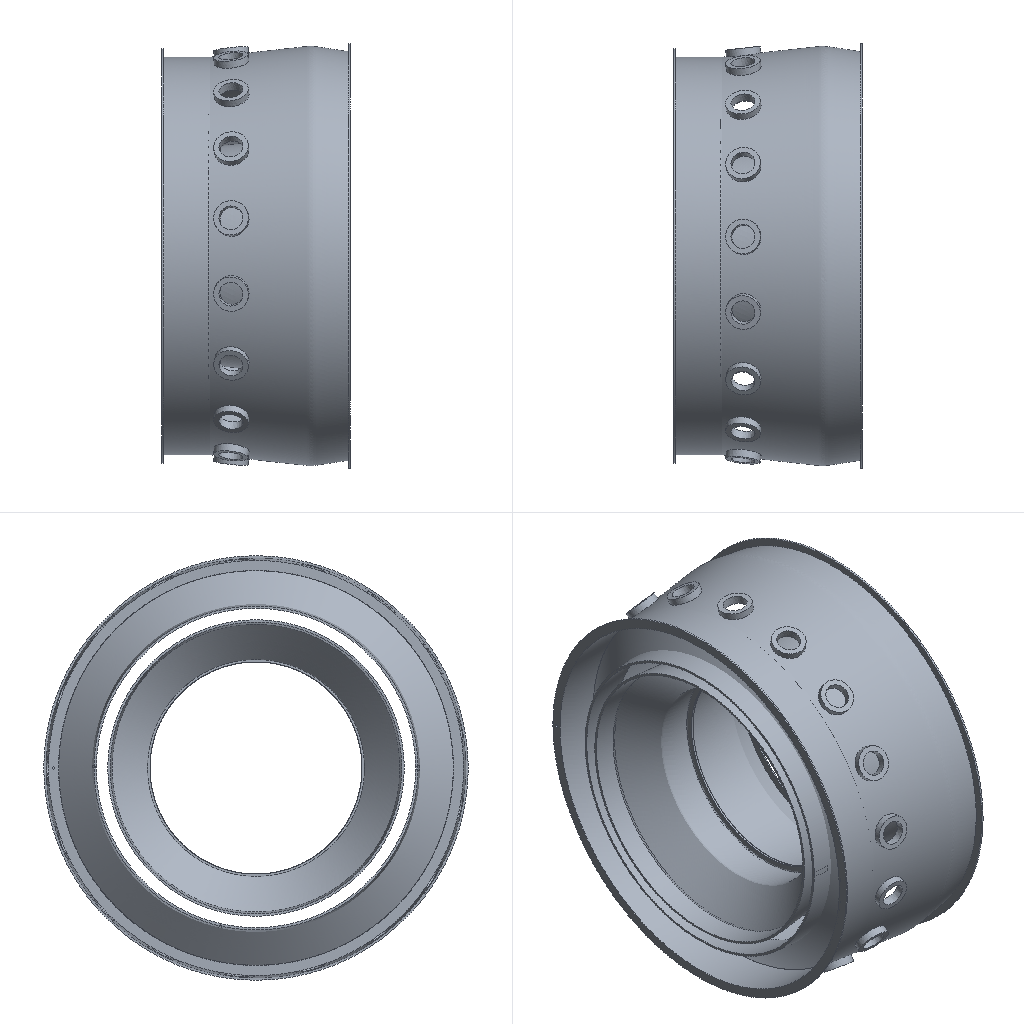Simulation study | ansys workbench
Set-up summary:
category,name,step,type,value,unit,region
solver,ansys_workbench
units,mm-N-s-tonne (MPa),,stated,"/units,MPA"
analysis,LS1,,steady-state thermal
load_step,LS1,LS1,steady-state thermal,nsubst=1; time=1
mesh,nodes,,,1043878
mesh,elements,,,772711
element_type,SOLID291,,,508745
element_type,SURF152,,,252830
element_type,SOLID279,,,6528
element_type,TARGE170,,,2304
element_type,CONTA174,,,2304
material,GH141,,E,216000
material,GH141,,nu,0.31
material,GH141,,density,8.27e-09,tonne mm^-3
material,GH141,,conductivity,8.37
material,GH141,,cte,1.054e-05
load,Define Uniform Initial temperature,model,body load temp,21.85,,all
load,"Create ""______""",LS1,convection,0.05,,SURF152 #8
load,"Create ""______ 2""",LS1,convection,0.288,,SURF152 #9
contact,Contact Region,,bonded (always),element=CONTA174
Ansys APDL input file, long lists of numbers shortened:
/batch
/config,noeldb,1     ! force off writing results to database
*get,_wallstrt,active,,time,wall
! ANSYS input file written by Workbench version 2021 R1
! File used for geometry attach:
/title,____+__+__--___ (B5)
! ****** Begin Custom Load Command Snippet ******
/COM, ACT Extensions:
/COM,     LSDYNA, 2021.1
/COM,
! ****** End   Custom Load Command Snippet ******
*DIM,_wb_ProjectScratch_dir,string,248
_wb_ProjectScratch_dir(1) = ''
*DIM,_wb_SolverFiles_dir,string,248
_wb_SolverFiles_dir(1) = ''
*DIM,_wb_userfiles_dir,string,248
_wb_userfiles_dir(1) = ''
/com,--- Data in consistent NMM units. See Solving Units in the help system for more information.
/units,MPA
/nopr
/wb,file,start              !  signify a WB generated input file
/prep7
! Turn off shape checking because checks already performed inside WB mesher.
! See help system for more information.
SHPP,OFF,,NOWARN
/nolist
etcon,set             ! allow ANSYS to choose best KEYOP's for 180x elements, resets any applicable keyopt to MAPDL defaults
/com,*********** Nodes for the whole assembly ***********
nblock,3,,1148263
(1i9,3e20.9e3)
        1    -2.909328663E+02    -6.564341511E+00     4.578700000E+02
! (1043875 more lines like these left out)
-1
/com,*********** Nodes for all Remote Points ***********
nblock,3
(1i9,3e20.9e3)
  1043877    -7.493286614E+01    -6.564353799E+00     2.143080415E+02
  1043878    -7.493286951E+01    -6.697121594E+00     2.143200000E+02
-1
/wb,elem,start            !  set before creation of elements
/com,*********** Elements for Body 1 "____9.24_\____9.24_" ***********
et,1,291
eblock,19,solid,,320859
(19i9)
        1        1        1        1        0        0        0        0       10        0   194415   420982   429274   496877   520848   545299   607590   545303   545309
! (641717 more lines like these left out)
-1
/com,*********** Elements for Body 2 "____0923_ (1)-0\____0923_ (1)" ***********
et,2,279
eblock,19,solid,,6528
(19i9)
        2        2        2        2        0        0        0        0       20        0        1     1050     1051    13262    13261     7008     7007    13469    13470
! (13055 more lines like these left out)
-1
/com,*********** Elements for Body 3 "______9.22_\______9.22_" ***********
et,3,291
eblock,19,solid,,92984
(19i9)
        3        3        3        3        0        0        0        0       10        0    35420    54545   103924   108327   107989   161558   401449   161564   161563
! (185967 more lines like these left out)
-1
/com,*********** Elements for Body 4 "______9.24_\______9.24_" ***********
et,4,291
eblock,19,solid,,66011
(19i9)
        4        4        3        4        0        0        0        0       10        0   128404    55040   108946   103353   108755   164427   399349   164424   164426
! (132021 more lines like these left out)
-1
/com,*********** Elements for Body 5 "____0923_ (1)\____0923_ (1)" ***********
et,5,291
eblock,19,solid,,28891
(19i9)
        5        5        3        5        0        0        0        0       10        0     6529    48274    97425   107256    48526   115927   382662   115929   115926
! (57781 more lines like these left out)
-1
/wb,elem,end               !  done creating elements
/com,*********** Send User Defined Coordinate System(s) ***********
csys,0
toffst,273.15,  ! Temperature offset from absolute zero
/wb,mat,start              !  starting to send materials
/com,*********** Send Materials ***********
Temperature = 'TEMP' ! Temperature
MP,DENS,1,8.27e-09,	! tonne mm^-3
MPTEMP,,,,,,,,
MPTEMP,1,100
MPTEMP,2,200
MPTEMP,3,300
MPTEMP,4,400
MPTEMP,5,500
MPTEMP,6,600
MPTEMP,7,700
MPTEMP,8,800
MPTEMP,9,900
MPDATA,EX,1, ,216000,210000,205000,200000,195000,188000,
MPDATA,EX,1, ,182000,175000,168000,	! tonne s^-2 mm^-1
MPTEMP,,,,,,,,
MPTEMP,,,,,,,,
MPTEMP,1,100
MPTEMP,2,200
MPTEMP,3,300
MPTEMP,4,400
MPTEMP,5,500
MPTEMP,6,600
MPTEMP,7,700
MPTEMP,8,800
MPTEMP,9,900
MPDATA,NUXY,1, ,0.31,0.31,0.31,0.31,0.31,0.31,
MPDATA,NUXY,1, ,0.31,0.31,0.31,
MPTEMP,,,,,,,,
MPTEMP,,,,,,,,
MPTEMP,1,100
MPTEMP,2,200
MPTEMP,3,300
MPTEMP,4,400
MPTEMP,5,500
MPTEMP,6,600
MPTEMP,7,700
MPTEMP,8,800
MPTEMP,9,900
MPDATA,ALPX,1, ,1.054e-05,1.169e-05,1.224e-05,1.278e-05,1.308e-05,1.348e-05,
MPDATA,ALPX,1, ,1.421e-05,1.497e-05,1.591e-05,	! C^-1
MPTEMP,,,,,,,,
MPTEMP,,,,,,,,
MPTEMP,1,100
MPTEMP,2,200
MPTEMP,3,300
MPTEMP,4,400
MPTEMP,5,500
MPTEMP,6,600
MPTEMP,7,700
MPTEMP,8,800
MPTEMP,9,900
MPDATA,KXX,1, ,8.37,10.47,12.56,15.07,17.17,19.56,
MPDATA,KXX,1, ,21.35,23.45,25.96,	! tonne mm s^-3 C^-1
MPTEMP,,,,,,,,
Temperature = 'TEMP' ! Temperature
MP,DENS,2,8.27e-09,	! tonne mm^-3
MPTEMP,,,,,,,,
MPTEMP,1,100
MPTEMP,2,200
MPTEMP,3,300
MPTEMP,4,400
MPTEMP,5,500
MPTEMP,6,600
MPTEMP,7,700
MPTEMP,8,800
MPTEMP,9,900
MPDATA,EX,2, ,216000,210000,205000,200000,195000,188000,
MPDATA,EX,2, ,182000,175000,168000,	! tonne s^-2 mm^-1
MPTEMP,,,,,,,,
MPTEMP,,,,,,,,
MPTEMP,1,100
MPTEMP,2,200
MPTEMP,3,300
MPTEMP,4,400
MPTEMP,5,500
MPTEMP,6,600
MPTEMP,7,700
MPTEMP,8,800
MPTEMP,9,900
MPDATA,NUXY,2, ,0.31,0.31,0.31,0.31,0.31,0.31,
MPDATA,NUXY,2, ,0.31,0.31,0.31,
MPTEMP,,,,,,,,
MPTEMP,,,,,,,,
MPTEMP,1,100
MPTEMP,2,200
MPTEMP,3,300
MPTEMP,4,400
MPTEMP,5,500
MPTEMP,6,600
MPTEMP,7,700
MPTEMP,8,800
MPTEMP,9,900
MPDATA,ALPX,2, ,1.054e-05,1.169e-05,1.224e-05,1.278e-05,1.308e-05,1.348e-05,
MPDATA,ALPX,2, ,1.421e-05,1.497e-05,1.591e-05,	! C^-1
MPTEMP,,,,,,,,
MPTEMP,,,,,,,,
MPTEMP,1,100
MPTEMP,2,200
MPTEMP,3,300
MPTEMP,4,400
MPTEMP,5,500
MPTEMP,6,600
MPTEMP,7,700
MPTEMP,8,800
MPTEMP,9,900
MPDATA,KXX,2, ,8.37,10.47,12.56,15.07,17.17,19.56,
MPDATA,KXX,2, ,21.35,23.45,25.96,	! tonne mm s^-3 C^-1
MPTEMP,,,,,,,,
Temperature = 'TEMP' ! Temperature
MP,DENS,3,8.27e-09,	! tonne mm^-3
MPTEMP,,,,,,,,
MPTEMP,1,100
MPTEMP,2,200
MPTEMP,3,300
MPTEMP,4,400
MPTEMP,5,500
MPTEMP,6,600
MPTEMP,7,700
MPTEMP,8,800
MPTEMP,9,900
MPDATA,EX,3, ,216000,210000,205000,200000,195000,188000,
MPDATA,EX,3, ,182000,175000,168000,	! tonne s^-2 mm^-1
MPTEMP,,,,,,,,
MPTEMP,,,,,,,,
MPTEMP,1,100
MPTEMP,2,200
MPTEMP,3,300
MPTEMP,4,400
MPTEMP,5,500
MPTEMP,6,600
MPTEMP,7,700
MPTEMP,8,800
MPTEMP,9,900
MPDATA,NUXY,3, ,0.31,0.31,0.31,0.31,0.31,0.31,
MPDATA,NUXY,3, ,0.31,0.31,0.31,
MPTEMP,,,,,,,,
MPTEMP,,,,,,,,
MPTEMP,1,100
MPTEMP,2,200
MPTEMP,3,300
MPTEMP,4,400
MPTEMP,5,500
MPTEMP,6,600
MPTEMP,7,700
MPTEMP,8,800
MPTEMP,9,900
MPDATA,ALPX,3, ,1.054e-05,1.169e-05,1.224e-05,1.278e-05,1.308e-05,1.348e-05,
MPDATA,ALPX,3, ,1.421e-05,1.497e-05,1.591e-05,	! C^-1
MPTEMP,,,,,,,,
MPTEMP,,,,,,,,
MPTEMP,1,100
MPTEMP,2,200
MPTEMP,3,300
MPTEMP,4,400
MPTEMP,5,500
MPTEMP,6,600
MPTEMP,7,700
MPTEMP,8,800
MPTEMP,9,900
MPDATA,KXX,3, ,8.37,10.47,12.56,15.07,17.17,19.56,
MPDATA,KXX,3, ,21.35,23.45,25.96,	! tonne mm s^-3 C^-1
MPTEMP,,,,,,,,
Temperature = 'TEMP' ! Temperature
MP,DENS,4,8.27e-09,	! tonne mm^-3
MPTEMP,,,,,,,,
MPTEMP,1,100
MPTEMP,2,200
MPTEMP,3,300
MPTEMP,4,400
MPTEMP,5,500
MPTEMP,6,600
MPTEMP,7,700
MPTEMP,8,800
MPTEMP,9,900
MPDATA,EX,4, ,216000,210000,205000,200000,195000,188000,
MPDATA,EX,4, ,182000,175000,168000,	! tonne s^-2 mm^-1
MPTEMP,,,,,,,,
MPTEMP,,,,,,,,
MPTEMP,1,100
MPTEMP,2,200
MPTEMP,3,300
MPTEMP,4,400
MPTEMP,5,500
MPTEMP,6,600
MPTEMP,7,700
MPTEMP,8,800
MPTEMP,9,900
MPDATA,NUXY,4, ,0.31,0.31,0.31,0.31,0.31,0.31,
MPDATA,NUXY,4, ,0.31,0.31,0.31,
MPTEMP,,,,,,,,
MPTEMP,,,,,,,,
MPTEMP,1,100
MPTEMP,2,200
MPTEMP,3,300
MPTEMP,4,400
MPTEMP,5,500
MPTEMP,6,600
MPTEMP,7,700
MPTEMP,8,800
MPTEMP,9,900
MPDATA,ALPX,4, ,1.054e-05,1.169e-05,1.224e-05,1.278e-05,1.308e-05,1.348e-05,
MPDATA,ALPX,4, ,1.421e-05,1.497e-05,1.591e-05,	! C^-1
MPTEMP,,,,,,,,
MPTEMP,,,,,,,,
MPTEMP,1,100
MPTEMP,2,200
MPTEMP,3,300
MPTEMP,4,400
MPTEMP,5,500
MPTEMP,6,600
MPTEMP,7,700
MPTEMP,8,800
MPTEMP,9,900
MPDATA,KXX,4, ,8.37,10.47,12.56,15.07,17.17,19.56,
MPDATA,KXX,4, ,21.35,23.45,25.96,	! tonne mm s^-3 C^-1
MPTEMP,,,,,,,,
Temperature = 'TEMP' ! Temperature
MP,DENS,5,8.27e-09,	! tonne mm^-3
MPTEMP,,,,,,,,
MPTEMP,1,100
MPTEMP,2,200
MPTEMP,3,300
MPTEMP,4,400
MPTEMP,5,500
MPTEMP,6,600
MPTEMP,7,700
MPTEMP,8,800
MPTEMP,9,900
MPDATA,EX,5, ,216000,210000,205000,200000,195000,188000,
MPDATA,EX,5, ,182000,175000,168000,	! tonne s^-2 mm^-1
MPTEMP,,,,,,,,
MPTEMP,,,,,,,,
MPTEMP,1,100
MPTEMP,2,200
MPTEMP,3,300
MPTEMP,4,400
MPTEMP,5,500
MPTEMP,6,600
MPTEMP,7,700
MPTEMP,8,800
MPTEMP,9,900
MPDATA,NUXY,5, ,0.31,0.31,0.31,0.31,0.31,0.31,
MPDATA,NUXY,5, ,0.31,0.31,0.31,
MPTEMP,,,,,,,,
MPTEMP,,,,,,,,
MPTEMP,1,100
MPTEMP,2,200
MPTEMP,3,300
MPTEMP,4,400
MPTEMP,5,500
MPTEMP,6,600
MPTEMP,7,700
MPTEMP,8,800
MPTEMP,9,900
MPDATA,ALPX,5, ,1.054e-05,1.169e-05,1.224e-05,1.278e-05,1.308e-05,1.348e-05,
MPDATA,ALPX,5, ,1.421e-05,1.497e-05,1.591e-05,	! C^-1
MPTEMP,,,,,,,,
MPTEMP,,,,,,,,
MPTEMP,1,100
MPTEMP,2,200
MPTEMP,3,300
MPTEMP,4,400
MPTEMP,5,500
MPTEMP,6,600
MPTEMP,7,700
MPTEMP,8,800
MPTEMP,9,900
MPDATA,KXX,5, ,8.37,10.47,12.56,15.07,17.17,19.56,
MPDATA,KXX,5, ,21.35,23.45,25.96,	! tonne mm s^-3 C^-1
MPTEMP,,,,,,,,
/wb,mat,end                !  done sending materials
!************************* Model Summary ********************
!____9.24_\____9.24_,	GH141,	matid,	1
!____0923_ (1)-0\____0923_ (1),	GH141,	matid,	2
!______9.22_\______9.22_,	GH141,	matid,	3
!______9.24_\______9.24_,	GH141,	matid,	4
!____0923_ (1)\____0923_ (1),	GH141,	matid,	5
!************************* End Model Summary ********************
! get the diagonal of the bounding box. Needed later for other things
*get,_xmin,node,,mnloc,x
*get,_ymin,node,,mnloc,y
*get,_zmin,node,,mnloc,z
*get,_xmax,node,,mxloc,x
*get,_ymax,node,,mxloc,y
*get,_zmax,node,,mxloc,z
_ASMDIAG=(_xmax-_xmin)*(_xmax-_xmin)+(_ymax-_ymin)*(_ymax-_ymin)+(_zmax-_zmin)*(_zmax-_zmin)
_ASMDIAG=SQRT(_ASMDIAG)
/wb,contact,start          !  starting to send contact
/com,*********** Create Contact "接触区域" ***********
/com,            Real Constant Set For Above Contact Is 7 & 6
*set,tid,7
*set,cid,6
r,tid
r,cid
et,tid,170
et,cid,174
eblock,10,,,768
(15i9)
   851572        7        7        7        0   423188   423189   423572   423572   564570   564576   423572   564572
! (767 more lines like these left out)
-1
eblock,10,,,768
(15i9)
   852340        6        6        6        0   423188   423189   423572   423572   564570   564576   423572   564572
! (767 more lines like these left out)
-1
eblock,10,,,1536
(15i9)
   853108        6        7        6        0     3446     3063     6901     6902    22949    22950    34083    24100
! (1535 more lines like these left out)
-1
eblock,10,,,1536
(15i9)
   854644        7        6        7        0     3446     3063     6901     6902    22949    22950    34083    24100
! (1535 more lines like these left out)
-1
keyo,cid,8,2               ! auto create asymmetric contact (from Program Controlled setting)
keyo,cid,10,0              ! adjust contact stiffness each NR iteration (from Program Controlled setting)
keyo,cid,12,5              ! bonded always
keyo,cid,18,1              ! small sliding turned on by application
keyo,cid,2,0               ! augmented Lagrange (from Program Controlled setting)
keyo,cid,4,0               ! on Gauss point (from Program Controlled setting)
keyo,cid,9,1               ! ignore initial gaps/penetration
keyo,cid,7,0               ! No Prediction
rmod,tid,3,10.      ! FKN
rmod,tid,5,0.       ! ICONT
rmod,tid,6,0.       ! PINB
rmod,tid,10,0.      ! CNOF
rmod,tid,12,0.      ! FKT
rmod,tid,36,113     ! WB DSID
rmod,cid,3,10.      ! FKN
rmod,cid,5,0.       ! ICONT
rmod,cid,6,0.       ! PINB
rmod,cid,10,0.      ! CNOF
rmod,cid,12,0.      ! FKT
rmod,cid,36,113     ! WB DSID
*set,_maxkxx,259600.
rmod,cid,14,_maxkxx/_ASMDIAG         ! TCC, Divide by Length since Traction Based
rmod,tid,14,_maxkxx/_ASMDIAG      ! TCC, Divide by Length since Traction Based
keyo,cid,1,2     ! Pure thermal contact
nsel,all
esel,all
/wb,contact,end            !  done creating contacts
/golist
/wb,load,start             !  starting to send loads
fcum,add                   ! add nodal forces up (needed in case have loads on the same edge,vertex)
fcum                       ! reset default on fcum command since done sending WB F loads
/com,*********** Create "______" ***********
et,8,152
eblock,10,,,132033
(15i9)
   856180        8        8        8        0   426206   426205   449370   449370   586312   586319   449370   586330
! (132032 more lines like these left out)
-1
esel,s,type,,8
keyop,8,8,2.
keyop,8,13,0
*DIM,_loadvari125,TABLE,2,1,1,TIME,
! Time values
_loadvari125(1,0,1) = 0.
_loadvari125(2,0,1) = 1.
! Load values
_loadvari125(1,1,1) = 486.85
_loadvari125(2,1,1) = 486.85
/com,*********** Create "______ 2" ***********
et,9,152
eblock,10,,,120797
(15i9)
   988213        9        9        9        0    51643    61963    61962    61962   141327   209382    61962   141326
! (120796 more lines like these left out)
-1
esel,s,type,,9
keyop,9,8,2.
keyop,9,13,0
*DIM,_loadvari127,TABLE,2,1,1,TIME,
! Time values
_loadvari127(1,0,1) = 0.
_loadvari127(2,0,1) = 1.
! Load values
_loadvari127(1,1,1) = 601.25
_loadvari127(2,1,1) = 601.25
esel,all
/com,***************** Define Uniform Initial temperature ***************
tunif,21.85
/gst,on,on
fini
*get,_numnode,node,0,count
*get,_numelem,elem,0,count
*get, _MAXELEMNUM, elem, 0, NUM, MAX
*get, _MAXNODENUM, node, 0, NUM, MAX
*get, _MAXELEMTYPE, etyp, 0, NUM, MAX
*get, _MAXREALCONST, real, 0, NUM, MAX
/go
/wb,load,end               !  done creating loads
/com,--- Number of total nodes = %_numnode%
/com,--- Number of contact elements = 257438
/com,--- Number of spring elements = 0
/com,--- Number of bearing elements = 0
/com,--- Number of solid elements = 515273
/com,--- Number of condensed parts = 0
/com,--- Number of total elements = %_numelem%
*get,_wallbsol,active,,time,wall
/com,****************************************************************************
/com,*************************    SOLUTION       ********************************
/com,****************************************************************************
/solu
antype,0                   ! static analysis
!eqsl,sparse               ! using sparse solver which is default so no eqsl command needed
cntr,print,1               ! print out contact info and also make no initial contact an error
rescontrol,,none                 ! Do not keep any restart files
dmpoption,emat,no             ! Don't combine emat file for DANSYS
dmpoption,esav,no             ! Don't combine esav file for DANSYS
/com,****************************************************
/com,******************* SOLVE FOR LS 1 OF 1 ****************
esel,s,type,,8
nsle
sf,all,conv,5.e-002,%_loadvari125%
esel,s,type,,9
nsle
sf,all,conv,0.288,%_loadvari127%
nsel,all
esel,all
autots,on
nsub,1,10,1
time,1.
outres,erase
outres,all,none
outres,nsol,all
outres,rsol,all
outres,eangl,all
outres,veng,all
outres,fflux,all
outres,cont,all
/nopr
esel,s,type,,8
esel,a,type,,9
cm,_elmisc,elem
esel,all
/gopr
outres,misc,all,_elmisc
cnvtol,heat,,.001,,1.e-003    ! Program Controlled. Set MINREF equivalent of 1e-6 Watts
! *********** WB SOLVE COMMAND ***********
! check interactive state
*get,ANSINTER_,active,,int
*if,ANSINTER_,ne,0,then
/eof
*endif
solve
/com *************** Write FE CONNECTORS *********
CEWRITE,file,ce,,INTE
/com,****************************************************
/com,*************** FINISHED SOLVE FOR LS 1 *************
*get,_wallasol,active,,time,wall
/post1
xmlo,ENCODING,ISO-8859-1
xmlo,parm
/xml,parm,xml
fini
/gopr
*get,_walldone,active,,time,wall
_preptime=(_wallbsol-_wallstrt)*3600
_solvtime=(_wallasol-_wallbsol)*3600
_posttime=(_walldone-_wallasol)*3600
_totaltim=(_walldone-_wallstrt)*3600
*get,_dlbratio,active,0,solu,dlbr
*get,_combtime,active,0,solu,comb
/com,--- Total number of nodes = %_numnode%
/com,--- Total number of elements = %_numelem%
/com,--- Element load balance ratio = %_dlbratio%
/com,--- Time to combine distributed files = %_combtime%
/wb,file,end               ! done with WB generated input
Results summary:
result,analyses[0].index,,,1
result,analyses[0].system,,,SYS-1
result,analyses[0].deck,,,deck.dat
result,analyses[0].solve_status,,,completed
result,analyses[0].analysis_type,,,static
result,analyses[0].physics,,,thermal
result,analyses[0].unit_system,,,"NMM: mm, ton, N, s, mV, mA, degC"
result,analyses[0].n_sets,,,1
result,analyses[0].load_steps[0].set,set=1,,1
result,analyses[0].load_steps[0].time_or_freq,set=1,,1
result,analyses[0].load_steps[0].max_temperature,set=1,,601.232
result,analyses[0].load_steps[0].min_temperature,set=1,,494.802
result,geometry_export[0][0],,,1.step
result,geometry_export[0][1],,,ok
result,geometry_export[0][2],,,39
result,geometry_export[1][0],,,2.step
result,geometry_export[1][1],,,ok
result,geometry_export[1][2],,,5